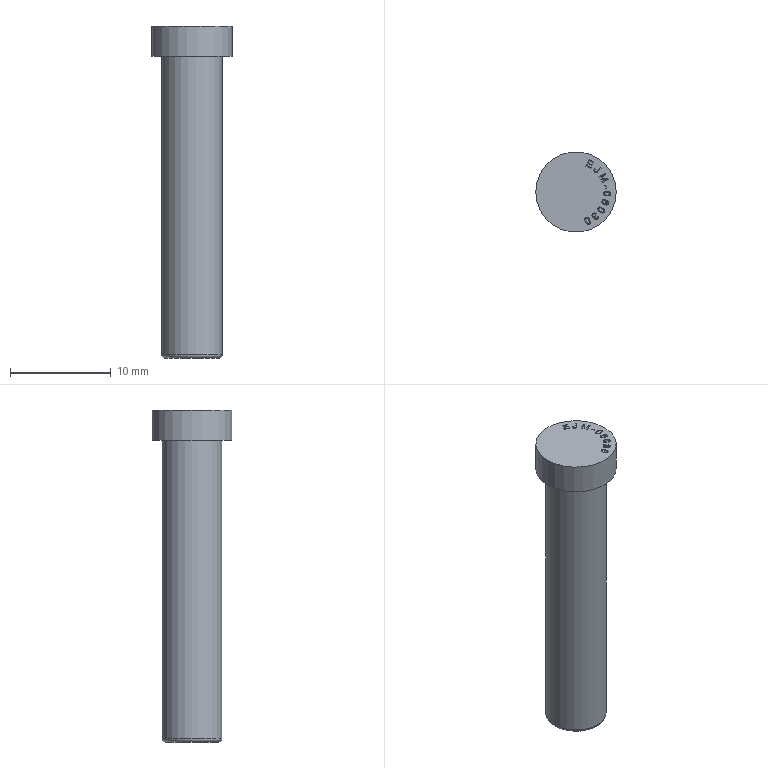Part | STEP file | lll_id2146_x_t | 1 solid | 81 faces | box 8 x 8 x 33 mm | volume 998.422 mm3 | plane 49 | other 29 | cylinder 2 | torus 1 | commonest cylinder face diameters 6 x1 8 x1